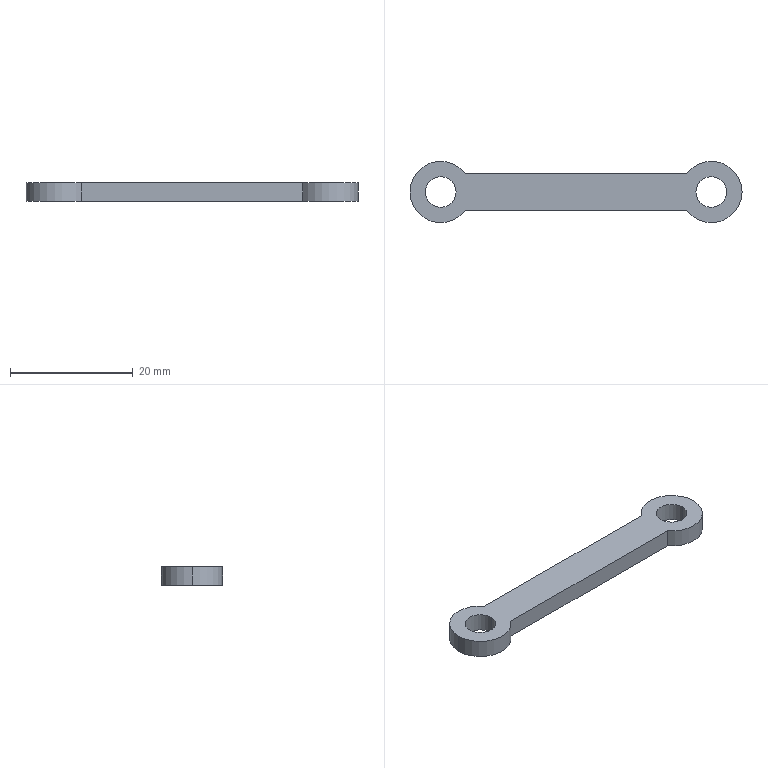Part | SolidWorks | features Extrusion 1 | 1 solid | 11 faces | box 54 x 10 x 3 mm | volume 976.904 mm3 | cylinder 7 | plane 4 | commonest cylinder face diameters 5 x4 10 x3
STEP:
#1=CARTESIAN_POINT('',(41.5,0.,3.));
#2=VERTEX_POINT('',#1);
#3=CARTESIAN_POINT('',(46.5,0.,3.));
#4=VERTEX_POINT('',#3);
#5=CARTESIAN_POINT('',(44.,0.,3.));
#6=DIRECTION('',(0.,0.,1.));
#7=DIRECTION('',(1.,0.,0.));
#8=AXIS2_PLACEMENT_3D('',#5,#6,#7);
#9=CIRCLE('',#8,2.5);
#10=EDGE_CURVE('',#2,#4,#9,.T.);
#11=ORIENTED_EDGE('',*,*,#10,.T.);
#12=CARTESIAN_POINT('',(46.5,0.,0.));
#13=VERTEX_POINT('',#12);
#14=CARTESIAN_POINT('',(46.5,0.,3.));
#15=DIRECTION('',(0.,0.,-1.));
#16=VECTOR('',#15,1000.);
#17=LINE('',#14,#16);
#18=EDGE_CURVE('',#4,#13,#17,.T.);
#19=ORIENTED_EDGE('',*,*,#18,.T.);
#20=CARTESIAN_POINT('',(41.5,0.,0.));
#21=VERTEX_POINT('',#20);
#22=CARTESIAN_POINT('',(44.,0.,0.));
#23=DIRECTION('',(0.,0.,1.));
#24=DIRECTION('',(1.,0.,0.));
#25=AXIS2_PLACEMENT_3D('',#22,#23,#24);
#26=CIRCLE('',#25,2.5);
#27=EDGE_CURVE('',#21,#13,#26,.T.);
#28=ORIENTED_EDGE('',*,*,#27,.F.);
#29=CARTESIAN_POINT('',(41.5,0.,3.));
#30=DIRECTION('',(0.,0.,-1.));
#31=VECTOR('',#30,1000.);
#32=LINE('',#29,#31);
#33=EDGE_CURVE('',#2,#21,#32,.T.);
#34=ORIENTED_EDGE('',*,*,#33,.F.);
#35=EDGE_LOOP('',(#11,#19,#28,#34));
#36=FACE_OUTER_BOUND('',#35,.T.);
#37=CARTESIAN_POINT('',(44.,0.,3.));
#38=DIRECTION('',(0.,0.,-1.));
#39=DIRECTION('',(-1.,0.,0.));
#40=AXIS2_PLACEMENT_3D('',#37,#38,#39);
#41=CYLINDRICAL_SURFACE('',#40,2.5);
#42=ADVANCED_FACE('',(#36),#41,.F.);
#43=CARTESIAN_POINT('',(-2.5,0.,3.));
#44=VERTEX_POINT('',#43);
#45=CARTESIAN_POINT('',(2.5,0.,3.));
#46=VERTEX_POINT('',#45);
#47=CARTESIAN_POINT('',(0.,0.,3.));
#48=DIRECTION('',(0.,0.,1.));
#49=DIRECTION('',(1.,0.,0.));
#50=AXIS2_PLACEMENT_3D('',#47,#48,#49);
#51=CIRCLE('',#50,2.5);
#52=EDGE_CURVE('',#44,#46,#51,.T.);
#53=ORIENTED_EDGE('',*,*,#52,.T.);
#54=CARTESIAN_POINT('',(2.5,0.,0.));
#55=VERTEX_POINT('',#54);
#56=CARTESIAN_POINT('',(2.5,0.,3.));
#57=DIRECTION('',(0.,0.,-1.));
#58=VECTOR('',#57,1000.);
#59=LINE('',#56,#58);
#60=EDGE_CURVE('',#46,#55,#59,.T.);
#61=ORIENTED_EDGE('',*,*,#60,.T.);
#62=CARTESIAN_POINT('',(-2.5,0.,0.));
#63=VERTEX_POINT('',#62);
#64=CARTESIAN_POINT('',(0.,0.,0.));
#65=DIRECTION('',(0.,0.,1.));
#66=DIRECTION('',(1.,0.,0.));
#67=AXIS2_PLACEMENT_3D('',#64,#65,#66);
#68=CIRCLE('',#67,2.5);
#69=EDGE_CURVE('',#63,#55,#68,.T.);
#70=ORIENTED_EDGE('',*,*,#69,.F.);
#71=CARTESIAN_POINT('',(-2.5,0.,3.));
#72=DIRECTION('',(0.,0.,-1.));
#73=VECTOR('',#72,1000.);
#74=LINE('',#71,#73);
#75=EDGE_CURVE('',#44,#63,#74,.T.);
#76=ORIENTED_EDGE('',*,*,#75,.F.);
#77=EDGE_LOOP('',(#53,#61,#70,#76));
#78=FACE_OUTER_BOUND('',#77,.T.);
#79=CARTESIAN_POINT('',(0.,0.,3.));
#80=DIRECTION('',(0.,0.,-1.));
#81=DIRECTION('',(-1.,0.,0.));
#82=AXIS2_PLACEMENT_3D('',#79,#80,#81);
#83=CYLINDRICAL_SURFACE('',#82,2.5);
#84=ADVANCED_FACE('',(#78),#83,.F.);
#85=CARTESIAN_POINT('',(-5.,0.,3.));
#86=VERTEX_POINT('',#85);
#87=CARTESIAN_POINT('',(4.,-3.,3.));
#88=VERTEX_POINT('',#87);
#89=CARTESIAN_POINT('',(0.,0.,3.));
#90=DIRECTION('',(0.,0.,1.));
#91=DIRECTION('',(1.,0.,0.));
#92=AXIS2_PLACEMENT_3D('',#89,#90,#91);
#93=CIRCLE('',#92,5.);
#94=EDGE_CURVE('',#86,#88,#93,.T.);
#95=ORIENTED_EDGE('',*,*,#94,.F.);
#96=CARTESIAN_POINT('',(-5.,0.,0.));
#97=VERTEX_POINT('',#96);
#98=CARTESIAN_POINT('',(-5.,0.,3.));
#99=DIRECTION('',(0.,0.,-1.));
#100=VECTOR('',#99,1000.);
#101=LINE('',#98,#100);
#102=EDGE_CURVE('',#86,#97,#101,.T.);
#103=ORIENTED_EDGE('',*,*,#102,.T.);
#104=CARTESIAN_POINT('',(4.,-3.,0.));
#105=VERTEX_POINT('',#104);
#106=CARTESIAN_POINT('',(0.,0.,0.));
#107=DIRECTION('',(0.,0.,1.));
#108=DIRECTION('',(1.,0.,0.));
#109=AXIS2_PLACEMENT_3D('',#106,#107,#108);
#110=CIRCLE('',#109,5.);
#111=EDGE_CURVE('',#97,#105,#110,.T.);
#112=ORIENTED_EDGE('',*,*,#111,.T.);
#113=CARTESIAN_POINT('',(4.,-3.,3.));
#114=DIRECTION('',(0.,0.,-1.));
#115=VECTOR('',#114,1000.);
#116=LINE('',#113,#115);
#117=EDGE_CURVE('',#88,#105,#116,.T.);
#118=ORIENTED_EDGE('',*,*,#117,.F.);
#119=EDGE_LOOP('',(#95,#103,#112,#118));
#120=FACE_OUTER_BOUND('',#119,.T.);
#121=CARTESIAN_POINT('',(0.,0.,3.));
#122=DIRECTION('',(0.,0.,-1.));
#123=DIRECTION('',(-1.,0.,0.));
#124=AXIS2_PLACEMENT_3D('',#121,#122,#123);
#125=CYLINDRICAL_SURFACE('',#124,5.);
#126=ADVANCED_FACE('',(#120),#125,.T.);
#127=ORIENTED_EDGE('',*,*,#52,.F.);
#128=CARTESIAN_POINT('',(0.,0.,3.));
#129=DIRECTION('',(0.,0.,1.));
#130=DIRECTION('',(1.,0.,0.));
#131=AXIS2_PLACEMENT_3D('',#128,#129,#130);
#132=CIRCLE('',#131,2.5);
#133=EDGE_CURVE('',#46,#44,#132,.T.);
#134=ORIENTED_EDGE('',*,*,#133,.F.);
#135=EDGE_LOOP('',(#127,#134));
#136=FACE_BOUND('',#135,.T.);
#137=CARTESIAN_POINT('',(40.,-3.,3.));
#138=VERTEX_POINT('',#137);
#139=CARTESIAN_POINT('',(40.,3.,3.));
#140=VERTEX_POINT('',#139);
#141=CARTESIAN_POINT('',(44.,0.,3.));
#142=DIRECTION('',(0.,0.,1.));
#143=DIRECTION('',(1.,0.,0.));
#144=AXIS2_PLACEMENT_3D('',#141,#142,#143);
#145=CIRCLE('',#144,5.);
#146=EDGE_CURVE('',#138,#140,#145,.T.);
#147=ORIENTED_EDGE('',*,*,#146,.T.);
#148=CARTESIAN_POINT('',(4.,3.,3.));
#149=VERTEX_POINT('',#148);
#150=CARTESIAN_POINT('',(4.,3.,3.));
#151=DIRECTION('',(-1.,0.,0.));
#152=VECTOR('',#151,1000.);
#153=LINE('',#150,#152);
#154=EDGE_CURVE('',#140,#149,#153,.T.);
#155=ORIENTED_EDGE('',*,*,#154,.T.);
#156=CARTESIAN_POINT('',(0.,0.,3.));
#157=DIRECTION('',(0.,0.,1.));
#158=DIRECTION('',(1.,0.,0.));
#159=AXIS2_PLACEMENT_3D('',#156,#157,#158);
#160=CIRCLE('',#159,5.);
#161=EDGE_CURVE('',#149,#86,#160,.T.);
#162=ORIENTED_EDGE('',*,*,#161,.T.);
#163=ORIENTED_EDGE('',*,*,#94,.T.);
#164=CARTESIAN_POINT('',(4.,-3.,3.));
#165=DIRECTION('',(1.,0.,0.));
#166=VECTOR('',#165,1000.);
#167=LINE('',#164,#166);
#168=EDGE_CURVE('',#88,#138,#167,.T.);
#169=ORIENTED_EDGE('',*,*,#168,.T.);
#170=EDGE_LOOP('',(#147,#155,#162,#163,#169));
#171=FACE_OUTER_BOUND('',#170,.T.);
#172=ORIENTED_EDGE('',*,*,#10,.F.);
#173=CARTESIAN_POINT('',(44.,0.,3.));
#174=DIRECTION('',(0.,0.,1.));
#175=DIRECTION('',(1.,0.,0.));
#176=AXIS2_PLACEMENT_3D('',#173,#174,#175);
#177=CIRCLE('',#176,2.5);
#178=EDGE_CURVE('',#4,#2,#177,.T.);
#179=ORIENTED_EDGE('',*,*,#178,.F.);
#180=EDGE_LOOP('',(#172,#179));
#181=FACE_BOUND('',#180,.T.);
#182=CARTESIAN_POINT('',(44.,0.,3.));
#183=DIRECTION('',(0.,0.,1.));
#184=DIRECTION('',(1.,0.,0.));
#185=AXIS2_PLACEMENT_3D('',#182,#183,#184);
#186=PLANE('',#185);
#187=ADVANCED_FACE('',(#136,#171,#181),#186,.T.);
#188=CARTESIAN_POINT('',(40.,-3.,0.));
#189=VERTEX_POINT('',#188);
#190=CARTESIAN_POINT('',(40.,3.,0.));
#191=VERTEX_POINT('',#190);
#192=CARTESIAN_POINT('',(44.,0.,0.));
#193=DIRECTION('',(0.,0.,1.));
#194=DIRECTION('',(1.,0.,0.));
#195=AXIS2_PLACEMENT_3D('',#192,#193,#194);
#196=CIRCLE('',#195,5.);
#197=EDGE_CURVE('',#189,#191,#196,.T.);
#198=ORIENTED_EDGE('',*,*,#197,.F.);
#199=CARTESIAN_POINT('',(4.,-3.,0.));
#200=DIRECTION('',(1.,0.,0.));
#201=VECTOR('',#200,1000.);
#202=LINE('',#199,#201);
#203=EDGE_CURVE('',#105,#189,#202,.T.);
#204=ORIENTED_EDGE('',*,*,#203,.F.);
#205=ORIENTED_EDGE('',*,*,#111,.F.);
#206=CARTESIAN_POINT('',(4.,3.,0.));
#207=VERTEX_POINT('',#206);
#208=CARTESIAN_POINT('',(0.,0.,0.));
#209=DIRECTION('',(0.,0.,1.));
#210=DIRECTION('',(1.,0.,0.));
#211=AXIS2_PLACEMENT_3D('',#208,#209,#210);
#212=CIRCLE('',#211,5.);
#213=EDGE_CURVE('',#207,#97,#212,.T.);
#214=ORIENTED_EDGE('',*,*,#213,.F.);
#215=CARTESIAN_POINT('',(4.,3.,0.));
#216=DIRECTION('',(-1.,0.,0.));
#217=VECTOR('',#216,1000.);
#218=LINE('',#215,#217);
#219=EDGE_CURVE('',#191,#207,#218,.T.);
#220=ORIENTED_EDGE('',*,*,#219,.F.);
#221=EDGE_LOOP('',(#198,#204,#205,#214,#220));
#222=FACE_OUTER_BOUND('',#221,.T.);
#223=ORIENTED_EDGE('',*,*,#69,.T.);
#224=CARTESIAN_POINT('',(0.,0.,0.));
#225=DIRECTION('',(0.,0.,1.));
#226=DIRECTION('',(1.,0.,0.));
#227=AXIS2_PLACEMENT_3D('',#224,#225,#226);
#228=CIRCLE('',#227,2.5);
#229=EDGE_CURVE('',#55,#63,#228,.T.);
#230=ORIENTED_EDGE('',*,*,#229,.T.);
#231=EDGE_LOOP('',(#223,#230));
#232=FACE_BOUND('',#231,.T.);
#233=ORIENTED_EDGE('',*,*,#27,.T.);
#234=CARTESIAN_POINT('',(44.,0.,0.));
#235=DIRECTION('',(0.,0.,1.));
#236=DIRECTION('',(1.,0.,0.));
#237=AXIS2_PLACEMENT_3D('',#234,#235,#236);
#238=CIRCLE('',#237,2.5);
#239=EDGE_CURVE('',#13,#21,#238,.T.);
#240=ORIENTED_EDGE('',*,*,#239,.T.);
#241=EDGE_LOOP('',(#233,#240));
#242=FACE_BOUND('',#241,.T.);
#243=CARTESIAN_POINT('',(44.,0.,0.));
#244=DIRECTION('',(0.,0.,1.));
#245=DIRECTION('',(1.,0.,0.));
#246=AXIS2_PLACEMENT_3D('',#243,#244,#245);
#247=PLANE('',#246);
#248=ADVANCED_FACE('',(#222,#232,#242),#247,.F.);
#249=ORIENTED_EDGE('',*,*,#197,.T.);
#250=CARTESIAN_POINT('',(40.,3.,3.));
#251=DIRECTION('',(0.,0.,-1.));
#252=VECTOR('',#251,1000.);
#253=LINE('',#250,#252);
#254=EDGE_CURVE('',#140,#191,#253,.T.);
#255=ORIENTED_EDGE('',*,*,#254,.F.);
#256=ORIENTED_EDGE('',*,*,#146,.F.);
#257=CARTESIAN_POINT('',(40.,-3.,3.));
#258=DIRECTION('',(0.,0.,-1.));
#259=VECTOR('',#258,1000.);
#260=LINE('',#257,#259);
#261=EDGE_CURVE('',#138,#189,#260,.T.);
#262=ORIENTED_EDGE('',*,*,#261,.T.);
#263=EDGE_LOOP('',(#249,#255,#256,#262));
#264=FACE_OUTER_BOUND('',#263,.T.);
#265=CARTESIAN_POINT('',(44.,0.,3.));
#266=DIRECTION('',(0.,0.,-1.));
#267=DIRECTION('',(-1.,0.,0.));
#268=AXIS2_PLACEMENT_3D('',#265,#266,#267);
#269=CYLINDRICAL_SURFACE('',#268,5.);
#270=ADVANCED_FACE('',(#264),#269,.T.);
#271=ORIENTED_EDGE('',*,*,#219,.T.);
#272=CARTESIAN_POINT('',(4.,3.,3.));
#273=DIRECTION('',(0.,0.,-1.));
#274=VECTOR('',#273,1000.);
#275=LINE('',#272,#274);
#276=EDGE_CURVE('',#149,#207,#275,.T.);
#277=ORIENTED_EDGE('',*,*,#276,.F.);
#278=ORIENTED_EDGE('',*,*,#154,.F.);
#279=ORIENTED_EDGE('',*,*,#254,.T.);
#280=EDGE_LOOP('',(#271,#277,#278,#279));
#281=FACE_OUTER_BOUND('',#280,.T.);
#282=CARTESIAN_POINT('',(4.,3.,3.));
#283=DIRECTION('',(0.,-1.,0.));
#284=DIRECTION('',(0.,0.,-1.));
#285=AXIS2_PLACEMENT_3D('',#282,#283,#284);
#286=PLANE('',#285);
#287=ADVANCED_FACE('',(#281),#286,.F.);
#288=ORIENTED_EDGE('',*,*,#102,.F.);
#289=ORIENTED_EDGE('',*,*,#161,.F.);
#290=ORIENTED_EDGE('',*,*,#276,.T.);
#291=ORIENTED_EDGE('',*,*,#213,.T.);
#292=EDGE_LOOP('',(#288,#289,#290,#291));
#293=FACE_OUTER_BOUND('',#292,.T.);
#294=CARTESIAN_POINT('',(0.,0.,3.));
#295=DIRECTION('',(0.,0.,-1.));
#296=DIRECTION('',(-1.,0.,0.));
#297=AXIS2_PLACEMENT_3D('',#294,#295,#296);
#298=CYLINDRICAL_SURFACE('',#297,5.);
#299=ADVANCED_FACE('',(#293),#298,.T.);
#300=ORIENTED_EDGE('',*,*,#203,.T.);
#301=ORIENTED_EDGE('',*,*,#261,.F.);
#302=ORIENTED_EDGE('',*,*,#168,.F.);
#303=ORIENTED_EDGE('',*,*,#117,.T.);
#304=EDGE_LOOP('',(#300,#301,#302,#303));
#305=FACE_OUTER_BOUND('',#304,.T.);
#306=CARTESIAN_POINT('',(4.,-3.,3.));
#307=DIRECTION('',(0.,1.,0.));
#308=DIRECTION('',(0.,0.,1.));
#309=AXIS2_PLACEMENT_3D('',#306,#307,#308);
#310=PLANE('',#309);
#311=ADVANCED_FACE('',(#305),#310,.F.);
#312=ORIENTED_EDGE('',*,*,#60,.F.);
#313=ORIENTED_EDGE('',*,*,#133,.T.);
#314=ORIENTED_EDGE('',*,*,#75,.T.);
#315=ORIENTED_EDGE('',*,*,#229,.F.);
#316=EDGE_LOOP('',(#312,#313,#314,#315));
#317=FACE_OUTER_BOUND('',#316,.T.);
#318=CARTESIAN_POINT('',(0.,0.,3.));
#319=DIRECTION('',(0.,0.,-1.));
#320=DIRECTION('',(-1.,0.,0.));
#321=AXIS2_PLACEMENT_3D('',#318,#319,#320);
#322=CYLINDRICAL_SURFACE('',#321,2.5);
#323=ADVANCED_FACE('',(#317),#322,.F.);
#324=ORIENTED_EDGE('',*,*,#18,.F.);
#325=ORIENTED_EDGE('',*,*,#178,.T.);
#326=ORIENTED_EDGE('',*,*,#33,.T.);
#327=ORIENTED_EDGE('',*,*,#239,.F.);
#328=EDGE_LOOP('',(#324,#325,#326,#327));
#329=FACE_OUTER_BOUND('',#328,.T.);
#330=CARTESIAN_POINT('',(44.,0.,3.));
#331=DIRECTION('',(0.,0.,-1.));
#332=DIRECTION('',(-1.,0.,0.));
#333=AXIS2_PLACEMENT_3D('',#330,#331,#332);
#334=CYLINDRICAL_SURFACE('',#333,2.5);
#335=ADVANCED_FACE('',(#329),#334,.F.);
#336=CLOSED_SHELL('',(#42,#84,#126,#187,#248,#270,#287,#299,#311,#323,#335));
#337=MANIFOLD_SOLID_BREP('',#336);
#338=CARTESIAN_POINT('',(0.,0.,0.));
#339=DIRECTION('',(0.,0.,1.));
#340=DIRECTION('',(1.,0.,0.));
#341=AXIS2_PLACEMENT_3D('',#338,#339,#340);
#342=(LENGTH_UNIT()NAMED_UNIT(*)SI_UNIT(.MILLI.,.METRE.));
#343=UNCERTAINTY_MEASURE_WITH_UNIT(LENGTH_MEASURE(0.00001),#342,'','');
#344=(NAMED_UNIT(*)PLANE_ANGLE_UNIT()SI_UNIT($,.RADIAN.));
#345=(NAMED_UNIT(*)SI_UNIT($,.STERADIAN.)SOLID_ANGLE_UNIT());
#346=(GEOMETRIC_REPRESENTATION_CONTEXT(3)GLOBAL_UNCERTAINTY_ASSIGNED_CONTEXT((#343))GLOBAL_UNIT_ASSIGNED_CONTEXT((#342,#344,#345))REPRESENTATION_CONTEXT('',''));
#347=ADVANCED_BREP_SHAPE_REPRESENTATION('',(#337,#341),#346);